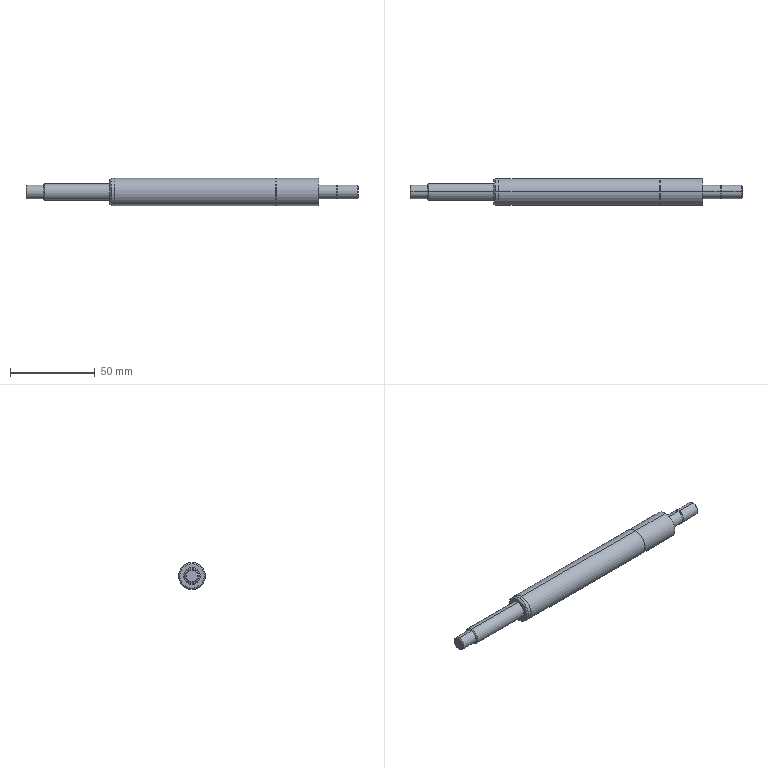Part | SolidWorks | features Chamfer 2, RevCut 1, Revolution 1 | 1 solid | 39 faces | box 196 x 16 x 16 mm | volume 29474 mm3 | cylinder 20 | plane 11 | cone 8 | commonest cylinder face diameters 8 x6 16 x6 12.8 x4 7.6 x2 10 x2
STEP:
#1=CARTESIAN_POINT('',(49.5,0.,7.2));
#2=VERTEX_POINT('',#1);
#3=CARTESIAN_POINT('',(49.5,0.,-7.2));
#4=VERTEX_POINT('',#3);
#5=CARTESIAN_POINT('',(49.5,0.,0.));
#6=DIRECTION('',(-1.,0.,0.));
#7=DIRECTION('',(0.,0.,1.));
#8=AXIS2_PLACEMENT_3D('',#5,#6,#7);
#9=CIRCLE('',#8,7.2);
#10=EDGE_CURVE('',#2,#4,#9,.T.);
#11=ORIENTED_EDGE('',*,*,#10,.F.);
#12=CARTESIAN_POINT('',(50.3,0.,8.));
#13=VERTEX_POINT('',#12);
#14=CARTESIAN_POINT('',(49.5,0.,7.2));
#15=DIRECTION('',(0.7071,0.,0.7071));
#16=VECTOR('',#15,1000.);
#17=LINE('',#14,#16);
#18=EDGE_CURVE('',#2,#13,#17,.T.);
#19=ORIENTED_EDGE('',*,*,#18,.T.);
#20=CARTESIAN_POINT('',(50.3,0.,-8.));
#21=VERTEX_POINT('',#20);
#22=CARTESIAN_POINT('',(50.3,0.,0.));
#23=DIRECTION('',(1.,0.,0.));
#24=DIRECTION('',(0.,0.,1.));
#25=AXIS2_PLACEMENT_3D('',#22,#23,#24);
#26=CIRCLE('',#25,8.);
#27=EDGE_CURVE('',#21,#13,#26,.T.);
#28=ORIENTED_EDGE('',*,*,#27,.F.);
#29=CARTESIAN_POINT('',(49.5,0.,-7.2));
#30=DIRECTION('',(0.7071,0.,-0.7071));
#31=VECTOR('',#30,1000.);
#32=LINE('',#29,#31);
#33=EDGE_CURVE('',#4,#21,#32,.T.);
#34=ORIENTED_EDGE('',*,*,#33,.F.);
#35=EDGE_LOOP('',(#11,#19,#28,#34));
#36=FACE_OUTER_BOUND('',#35,.T.);
#37=CARTESIAN_POINT('',(49.5,0.,0.));
#38=DIRECTION('',(1.,0.,0.));
#39=DIRECTION('',(0.,0.,-1.));
#40=AXIS2_PLACEMENT_3D('',#37,#38,#39);
#41=CONICAL_SURFACE('',#40,7.2,0.7854);
#42=ADVANCED_FACE('',(#36),#41,.T.);
#43=CARTESIAN_POINT('',(196.,0.,-3.5));
#44=VERTEX_POINT('',#43);
#45=CARTESIAN_POINT('',(196.,0.,3.5));
#46=VERTEX_POINT('',#45);
#47=CARTESIAN_POINT('',(196.,0.,0.));
#48=DIRECTION('',(1.,0.,0.));
#49=DIRECTION('',(0.,0.,-1.));
#50=AXIS2_PLACEMENT_3D('',#47,#48,#49);
#51=CIRCLE('',#50,3.5);
#52=EDGE_CURVE('',#44,#46,#51,.T.);
#53=ORIENTED_EDGE('',*,*,#52,.F.);
#54=CARTESIAN_POINT('',(195.5,0.,-4.));
#55=VERTEX_POINT('',#54);
#56=CARTESIAN_POINT('',(195.5,0.,-4.));
#57=DIRECTION('',(-0.7071,0.,-0.7071));
#58=VECTOR('',#57,1000.);
#59=LINE('',#56,#58);
#60=EDGE_CURVE('',#44,#55,#59,.T.);
#61=ORIENTED_EDGE('',*,*,#60,.T.);
#62=CARTESIAN_POINT('',(195.5,0.,4.));
#63=VERTEX_POINT('',#62);
#64=CARTESIAN_POINT('',(195.5,0.,0.));
#65=DIRECTION('',(-1.,0.,0.));
#66=DIRECTION('',(0.,0.,-1.));
#67=AXIS2_PLACEMENT_3D('',#64,#65,#66);
#68=CIRCLE('',#67,4.);
#69=EDGE_CURVE('',#63,#55,#68,.T.);
#70=ORIENTED_EDGE('',*,*,#69,.F.);
#71=CARTESIAN_POINT('',(195.5,0.,4.));
#72=DIRECTION('',(-0.7071,0.,0.7071));
#73=VECTOR('',#72,1000.);
#74=LINE('',#71,#73);
#75=EDGE_CURVE('',#46,#63,#74,.T.);
#76=ORIENTED_EDGE('',*,*,#75,.F.);
#77=EDGE_LOOP('',(#53,#61,#70,#76));
#78=FACE_OUTER_BOUND('',#77,.T.);
#79=CARTESIAN_POINT('',(195.5,0.,0.));
#80=DIRECTION('',(-1.,0.,0.));
#81=DIRECTION('',(0.,0.,1.));
#82=AXIS2_PLACEMENT_3D('',#79,#80,#81);
#83=CONICAL_SURFACE('',#82,4.,0.7854);
#84=ADVANCED_FACE('',(#78),#83,.T.);
#85=CARTESIAN_POINT('',(0.,0.,3.5));
#86=VERTEX_POINT('',#85);
#87=CARTESIAN_POINT('',(0.,0.,-3.5));
#88=VERTEX_POINT('',#87);
#89=CARTESIAN_POINT('',(0.,0.,0.));
#90=DIRECTION('',(-1.,0.,0.));
#91=DIRECTION('',(0.,0.,1.));
#92=AXIS2_PLACEMENT_3D('',#89,#90,#91);
#93=CIRCLE('',#92,3.5);
#94=EDGE_CURVE('',#86,#88,#93,.T.);
#95=ORIENTED_EDGE('',*,*,#94,.F.);
#96=CARTESIAN_POINT('',(0.5,0.,4.));
#97=VERTEX_POINT('',#96);
#98=CARTESIAN_POINT('',(0.,0.,3.5));
#99=DIRECTION('',(0.7071,0.,0.7071));
#100=VECTOR('',#99,1000.);
#101=LINE('',#98,#100);
#102=EDGE_CURVE('',#86,#97,#101,.T.);
#103=ORIENTED_EDGE('',*,*,#102,.T.);
#104=CARTESIAN_POINT('',(0.5,0.,-4.));
#105=VERTEX_POINT('',#104);
#106=CARTESIAN_POINT('',(0.5,0.,0.));
#107=DIRECTION('',(1.,0.,0.));
#108=DIRECTION('',(0.,0.,1.));
#109=AXIS2_PLACEMENT_3D('',#106,#107,#108);
#110=CIRCLE('',#109,4.);
#111=EDGE_CURVE('',#105,#97,#110,.T.);
#112=ORIENTED_EDGE('',*,*,#111,.F.);
#113=CARTESIAN_POINT('',(0.,0.,-3.5));
#114=DIRECTION('',(0.7071,0.,-0.7071));
#115=VECTOR('',#114,1000.);
#116=LINE('',#113,#115);
#117=EDGE_CURVE('',#88,#105,#116,.T.);
#118=ORIENTED_EDGE('',*,*,#117,.F.);
#119=EDGE_LOOP('',(#95,#103,#112,#118));
#120=FACE_OUTER_BOUND('',#119,.T.);
#121=CARTESIAN_POINT('',(0.,0.,0.));
#122=DIRECTION('',(1.,0.,0.));
#123=DIRECTION('',(0.,0.,-1.));
#124=AXIS2_PLACEMENT_3D('',#121,#122,#123);
#125=CONICAL_SURFACE('',#124,3.5,0.7854);
#126=ADVANCED_FACE('',(#120),#125,.T.);
#127=CARTESIAN_POINT('',(10.5,0.,4.5));
#128=VERTEX_POINT('',#127);
#129=CARTESIAN_POINT('',(10.5,0.,-4.5));
#130=VERTEX_POINT('',#129);
#131=CARTESIAN_POINT('',(10.5,0.,0.));
#132=DIRECTION('',(-1.,0.,0.));
#133=DIRECTION('',(0.,0.,1.));
#134=AXIS2_PLACEMENT_3D('',#131,#132,#133);
#135=CIRCLE('',#134,4.5);
#136=EDGE_CURVE('',#128,#130,#135,.T.);
#137=ORIENTED_EDGE('',*,*,#136,.F.);
#138=CARTESIAN_POINT('',(11.,0.,5.));
#139=VERTEX_POINT('',#138);
#140=CARTESIAN_POINT('',(10.5,0.,4.5));
#141=DIRECTION('',(0.7071,0.,0.7071));
#142=VECTOR('',#141,1000.);
#143=LINE('',#140,#142);
#144=EDGE_CURVE('',#128,#139,#143,.T.);
#145=ORIENTED_EDGE('',*,*,#144,.T.);
#146=CARTESIAN_POINT('',(11.,0.,-5.));
#147=VERTEX_POINT('',#146);
#148=CARTESIAN_POINT('',(11.,0.,0.));
#149=DIRECTION('',(1.,0.,0.));
#150=DIRECTION('',(0.,0.,1.));
#151=AXIS2_PLACEMENT_3D('',#148,#149,#150);
#152=CIRCLE('',#151,5.);
#153=EDGE_CURVE('',#147,#139,#152,.T.);
#154=ORIENTED_EDGE('',*,*,#153,.F.);
#155=CARTESIAN_POINT('',(10.5,0.,-4.5));
#156=DIRECTION('',(0.7071,0.,-0.7071));
#157=VECTOR('',#156,1000.);
#158=LINE('',#155,#157);
#159=EDGE_CURVE('',#130,#147,#158,.T.);
#160=ORIENTED_EDGE('',*,*,#159,.F.);
#161=EDGE_LOOP('',(#137,#145,#154,#160));
#162=FACE_OUTER_BOUND('',#161,.T.);
#163=CARTESIAN_POINT('',(10.5,0.,0.));
#164=DIRECTION('',(1.,0.,0.));
#165=DIRECTION('',(0.,0.,-1.));
#166=AXIS2_PLACEMENT_3D('',#163,#164,#165);
#167=CONICAL_SURFACE('',#166,4.5,0.7854);
#168=ADVANCED_FACE('',(#162),#167,.T.);
#169=ORIENTED_EDGE('',*,*,#69,.T.);
#170=CARTESIAN_POINT('',(184.,0.,-4.));
#171=VERTEX_POINT('',#170);
#172=CARTESIAN_POINT('',(-12.257,0.,-4.));
#173=DIRECTION('',(-1.,0.,0.));
#174=VECTOR('',#173,1000.);
#175=LINE('',#172,#174);
#176=EDGE_CURVE('',#55,#171,#175,.T.);
#177=ORIENTED_EDGE('',*,*,#176,.T.);
#178=CARTESIAN_POINT('',(184.,0.,4.));
#179=VERTEX_POINT('',#178);
#180=CARTESIAN_POINT('',(184.,0.,0.));
#181=DIRECTION('',(-1.,0.,0.));
#182=DIRECTION('',(0.,0.,1.));
#183=AXIS2_PLACEMENT_3D('',#180,#181,#182);
#184=CIRCLE('',#183,4.);
#185=EDGE_CURVE('',#179,#171,#184,.T.);
#186=ORIENTED_EDGE('',*,*,#185,.F.);
#187=CARTESIAN_POINT('',(-12.257,0.,4.));
#188=DIRECTION('',(-1.,0.,0.));
#189=VECTOR('',#188,1000.);
#190=LINE('',#187,#189);
#191=EDGE_CURVE('',#63,#179,#190,.T.);
#192=ORIENTED_EDGE('',*,*,#191,.F.);
#193=EDGE_LOOP('',(#169,#177,#186,#192));
#194=FACE_OUTER_BOUND('',#193,.T.);
#195=CARTESIAN_POINT('',(-12.257,0.,0.));
#196=DIRECTION('',(-1.,0.,0.));
#197=DIRECTION('',(0.,0.,1.));
#198=AXIS2_PLACEMENT_3D('',#195,#196,#197);
#199=CYLINDRICAL_SURFACE('',#198,4.);
#200=ADVANCED_FACE('',(#194),#199,.T.);
#201=CARTESIAN_POINT('',(184.,0.,3.8));
#202=VERTEX_POINT('',#201);
#203=CARTESIAN_POINT('',(184.,0.,-3.8));
#204=VERTEX_POINT('',#203);
#205=CARTESIAN_POINT('',(184.,0.,0.));
#206=DIRECTION('',(-1.,0.,0.));
#207=DIRECTION('',(0.,0.,1.));
#208=AXIS2_PLACEMENT_3D('',#205,#206,#207);
#209=CIRCLE('',#208,3.8);
#210=EDGE_CURVE('',#202,#204,#209,.T.);
#211=ORIENTED_EDGE('',*,*,#210,.T.);
#212=CARTESIAN_POINT('',(183.1,0.,-3.8));
#213=VERTEX_POINT('',#212);
#214=CARTESIAN_POINT('',(-6.355,0.,-3.8));
#215=DIRECTION('',(-1.,0.,0.));
#216=VECTOR('',#215,1000.);
#217=LINE('',#214,#216);
#218=EDGE_CURVE('',#204,#213,#217,.T.);
#219=ORIENTED_EDGE('',*,*,#218,.T.);
#220=CARTESIAN_POINT('',(183.1,0.,3.8));
#221=VERTEX_POINT('',#220);
#222=CARTESIAN_POINT('',(183.1,0.,0.));
#223=DIRECTION('',(-1.,0.,0.));
#224=DIRECTION('',(0.,0.,1.));
#225=AXIS2_PLACEMENT_3D('',#222,#223,#224);
#226=CIRCLE('',#225,3.8);
#227=EDGE_CURVE('',#221,#213,#226,.T.);
#228=ORIENTED_EDGE('',*,*,#227,.F.);
#229=CARTESIAN_POINT('',(-6.355,0.,3.8));
#230=DIRECTION('',(-1.,0.,0.));
#231=VECTOR('',#230,1000.);
#232=LINE('',#229,#231);
#233=EDGE_CURVE('',#202,#221,#232,.T.);
#234=ORIENTED_EDGE('',*,*,#233,.F.);
#235=EDGE_LOOP('',(#211,#219,#228,#234));
#236=FACE_OUTER_BOUND('',#235,.T.);
#237=CARTESIAN_POINT('',(-6.355,0.,0.));
#238=DIRECTION('',(-1.,0.,0.));
#239=DIRECTION('',(0.,0.,1.));
#240=AXIS2_PLACEMENT_3D('',#237,#238,#239);
#241=CYLINDRICAL_SURFACE('',#240,3.8);
#242=ADVANCED_FACE('',(#236),#241,.T.);
#243=CARTESIAN_POINT('',(172.7,0.,8.));
#244=VERTEX_POINT('',#243);
#245=CARTESIAN_POINT('',(172.7,0.,-8.));
#246=VERTEX_POINT('',#245);
#247=CARTESIAN_POINT('',(172.7,0.,0.));
#248=DIRECTION('',(-1.,0.,0.));
#249=DIRECTION('',(0.,0.,1.));
#250=AXIS2_PLACEMENT_3D('',#247,#248,#249);
#251=CIRCLE('',#250,8.);
#252=EDGE_CURVE('',#244,#246,#251,.T.);
#253=ORIENTED_EDGE('',*,*,#252,.T.);
#254=CARTESIAN_POINT('',(147.7,0.,-8.));
#255=VERTEX_POINT('',#254);
#256=CARTESIAN_POINT('',(-12.257,0.,-8.));
#257=DIRECTION('',(-1.,0.,0.));
#258=VECTOR('',#257,1000.);
#259=LINE('',#256,#258);
#260=EDGE_CURVE('',#246,#255,#259,.T.);
#261=ORIENTED_EDGE('',*,*,#260,.T.);
#262=CARTESIAN_POINT('',(147.7,0.,8.));
#263=VERTEX_POINT('',#262);
#264=CARTESIAN_POINT('',(147.7,0.,0.));
#265=DIRECTION('',(-1.,0.,0.));
#266=DIRECTION('',(0.,0.,1.));
#267=AXIS2_PLACEMENT_3D('',#264,#265,#266);
#268=CIRCLE('',#267,8.);
#269=EDGE_CURVE('',#263,#255,#268,.T.);
#270=ORIENTED_EDGE('',*,*,#269,.F.);
#271=CARTESIAN_POINT('',(-12.257,0.,8.));
#272=DIRECTION('',(-1.,0.,0.));
#273=VECTOR('',#272,1000.);
#274=LINE('',#271,#273);
#275=EDGE_CURVE('',#244,#263,#274,.T.);
#276=ORIENTED_EDGE('',*,*,#275,.F.);
#277=EDGE_LOOP('',(#253,#261,#270,#276));
#278=FACE_OUTER_BOUND('',#277,.T.);
#279=CARTESIAN_POINT('',(-12.257,0.,0.));
#280=DIRECTION('',(-1.,0.,0.));
#281=DIRECTION('',(0.,0.,1.));
#282=AXIS2_PLACEMENT_3D('',#279,#280,#281);
#283=CYLINDRICAL_SURFACE('',#282,8.);
#284=ADVANCED_FACE('',(#278),#283,.T.);
#285=CARTESIAN_POINT('',(147.7,0.,6.4));
#286=VERTEX_POINT('',#285);
#287=CARTESIAN_POINT('',(147.7,0.,-6.4));
#288=VERTEX_POINT('',#287);
#289=CARTESIAN_POINT('',(147.7,0.,0.));
#290=DIRECTION('',(-1.,0.,0.));
#291=DIRECTION('',(0.,0.,1.));
#292=AXIS2_PLACEMENT_3D('',#289,#290,#291);
#293=CIRCLE('',#292,6.4);
#294=EDGE_CURVE('',#286,#288,#293,.T.);
#295=ORIENTED_EDGE('',*,*,#294,.T.);
#296=CARTESIAN_POINT('',(147.5,0.,-6.4));
#297=VERTEX_POINT('',#296);
#298=CARTESIAN_POINT('',(-6.355,0.,-6.4));
#299=DIRECTION('',(-1.,0.,0.));
#300=VECTOR('',#299,1000.);
#301=LINE('',#298,#300);
#302=EDGE_CURVE('',#288,#297,#301,.T.);
#303=ORIENTED_EDGE('',*,*,#302,.T.);
#304=CARTESIAN_POINT('',(147.5,0.,6.4));
#305=VERTEX_POINT('',#304);
#306=CARTESIAN_POINT('',(147.5,0.,0.));
#307=DIRECTION('',(-1.,0.,0.));
#308=DIRECTION('',(0.,0.,1.));
#309=AXIS2_PLACEMENT_3D('',#306,#307,#308);
#310=CIRCLE('',#309,6.4);
#311=EDGE_CURVE('',#305,#297,#310,.T.);
#312=ORIENTED_EDGE('',*,*,#311,.F.);
#313=CARTESIAN_POINT('',(-6.355,0.,6.4));
#314=DIRECTION('',(-1.,0.,0.));
#315=VECTOR('',#314,1000.);
#316=LINE('',#313,#315);
#317=EDGE_CURVE('',#286,#305,#316,.T.);
#318=ORIENTED_EDGE('',*,*,#317,.F.);
#319=EDGE_LOOP('',(#295,#303,#312,#318));
#320=FACE_OUTER_BOUND('',#319,.T.);
#321=CARTESIAN_POINT('',(-6.355,0.,0.));
#322=DIRECTION('',(-1.,0.,0.));
#323=DIRECTION('',(0.,0.,1.));
#324=AXIS2_PLACEMENT_3D('',#321,#322,#323);
#325=CYLINDRICAL_SURFACE('',#324,6.4);
#326=ADVANCED_FACE('',(#320),#325,.T.);
#327=CARTESIAN_POINT('',(52.5,0.,6.4));
#328=VERTEX_POINT('',#327);
#329=CARTESIAN_POINT('',(52.5,0.,-6.4));
#330=VERTEX_POINT('',#329);
#331=CARTESIAN_POINT('',(52.5,0.,0.));
#332=DIRECTION('',(-1.,0.,0.));
#333=DIRECTION('',(0.,0.,1.));
#334=AXIS2_PLACEMENT_3D('',#331,#332,#333);
#335=CIRCLE('',#334,6.4);
#336=EDGE_CURVE('',#328,#330,#335,.T.);
#337=ORIENTED_EDGE('',*,*,#336,.T.);
#338=CARTESIAN_POINT('',(52.3,0.,-6.4));
#339=VERTEX_POINT('',#338);
#340=CARTESIAN_POINT('',(-6.355,0.,-6.4));
#341=DIRECTION('',(-1.,0.,0.));
#342=VECTOR('',#341,1000.);
#343=LINE('',#340,#342);
#344=EDGE_CURVE('',#330,#339,#343,.T.);
#345=ORIENTED_EDGE('',*,*,#344,.T.);
#346=CARTESIAN_POINT('',(52.3,0.,6.4));
#347=VERTEX_POINT('',#346);
#348=CARTESIAN_POINT('',(52.3,0.,0.));
#349=DIRECTION('',(-1.,0.,0.));
#350=DIRECTION('',(0.,0.,1.));
#351=AXIS2_PLACEMENT_3D('',#348,#349,#350);
#352=CIRCLE('',#351,6.4);
#353=EDGE_CURVE('',#347,#339,#352,.T.);
#354=ORIENTED_EDGE('',*,*,#353,.F.);
#355=CARTESIAN_POINT('',(-6.355,0.,6.4));
#356=DIRECTION('',(-1.,0.,0.));
#357=VECTOR('',#356,1000.);
#358=LINE('',#355,#357);
#359=EDGE_CURVE('',#328,#347,#358,.T.);
#360=ORIENTED_EDGE('',*,*,#359,.F.);
#361=EDGE_LOOP('',(#337,#345,#354,#360));
#362=FACE_OUTER_BOUND('',#361,.T.);
#363=CARTESIAN_POINT('',(-6.355,0.,0.));
#364=DIRECTION('',(-1.,0.,0.));
#365=DIRECTION('',(0.,0.,1.));
#366=AXIS2_PLACEMENT_3D('',#363,#364,#365);
#367=CYLINDRICAL_SURFACE('',#366,6.4);
#368=ADVANCED_FACE('',(#362),#367,.T.);
#369=CARTESIAN_POINT('',(49.5,0.,5.));
#370=VERTEX_POINT('',#369);
#371=CARTESIAN_POINT('',(49.5,0.,-5.));
#372=VERTEX_POINT('',#371);
#373=CARTESIAN_POINT('',(49.5,0.,0.));
#374=DIRECTION('',(-1.,0.,0.));
#375=DIRECTION('',(0.,0.,1.));
#376=AXIS2_PLACEMENT_3D('',#373,#374,#375);
#377=CIRCLE('',#376,5.);
#378=EDGE_CURVE('',#370,#372,#377,.T.);
#379=ORIENTED_EDGE('',*,*,#378,.T.);
#380=CARTESIAN_POINT('',(-12.257,0.,-5.));
#381=DIRECTION('',(-1.,0.,0.));
#382=VECTOR('',#381,1000.);
#383=LINE('',#380,#382);
#384=EDGE_CURVE('',#372,#147,#383,.T.);
#385=ORIENTED_EDGE('',*,*,#384,.T.);
#386=ORIENTED_EDGE('',*,*,#153,.T.);
#387=CARTESIAN_POINT('',(-12.257,0.,5.));
#388=DIRECTION('',(-1.,0.,0.));
#389=VECTOR('',#388,1000.);
#390=LINE('',#387,#389);
#391=EDGE_CURVE('',#370,#139,#390,.T.);
#392=ORIENTED_EDGE('',*,*,#391,.F.);
#393=EDGE_LOOP('',(#379,#385,#386,#392));
#394=FACE_OUTER_BOUND('',#393,.T.);
#395=CARTESIAN_POINT('',(-12.257,0.,0.));
#396=DIRECTION('',(-1.,0.,0.));
#397=DIRECTION('',(0.,0.,1.));
#398=AXIS2_PLACEMENT_3D('',#395,#396,#397);
#399=CYLINDRICAL_SURFACE('',#398,5.);
#400=ADVANCED_FACE('',(#394),#399,.T.);
#401=CARTESIAN_POINT('',(10.5,0.,4.));
#402=VERTEX_POINT('',#401);
#403=CARTESIAN_POINT('',(10.5,0.,-4.));
#404=VERTEX_POINT('',#403);
#405=CARTESIAN_POINT('',(10.5,0.,0.));
#406=DIRECTION('',(-1.,0.,0.));
#407=DIRECTION('',(0.,0.,1.));
#408=AXIS2_PLACEMENT_3D('',#405,#406,#407);
#409=CIRCLE('',#408,4.);
#410=EDGE_CURVE('',#402,#404,#409,.T.);
#411=ORIENTED_EDGE('',*,*,#410,.T.);
#412=CARTESIAN_POINT('',(-12.257,0.,-4.));
#413=DIRECTION('',(-1.,0.,0.));
#414=VECTOR('',#413,1000.);
#415=LINE('',#412,#414);
#416=EDGE_CURVE('',#404,#105,#415,.T.);
#417=ORIENTED_EDGE('',*,*,#416,.T.);
#418=ORIENTED_EDGE('',*,*,#111,.T.);
#419=CARTESIAN_POINT('',(-12.257,0.,4.));
#420=DIRECTION('',(-1.,0.,0.));
#421=VECTOR('',#420,1000.);
#422=LINE('',#419,#421);
#423=EDGE_CURVE('',#402,#97,#422,.T.);
#424=ORIENTED_EDGE('',*,*,#423,.F.);
#425=EDGE_LOOP('',(#411,#417,#418,#424));
#426=FACE_OUTER_BOUND('',#425,.T.);
#427=CARTESIAN_POINT('',(-12.257,0.,0.));
#428=DIRECTION('',(-1.,0.,0.));
#429=DIRECTION('',(0.,0.,1.));
#430=AXIS2_PLACEMENT_3D('',#427,#428,#429);
#431=CYLINDRICAL_SURFACE('',#430,4.);
#432=ADVANCED_FACE('',(#426),#431,.T.);
#433=CARTESIAN_POINT('',(52.3,0.,8.));
#434=VERTEX_POINT('',#433);
#435=CARTESIAN_POINT('',(52.3,0.,-8.));
#436=VERTEX_POINT('',#435);
#437=CARTESIAN_POINT('',(52.3,0.,0.));
#438=DIRECTION('',(-1.,0.,0.));
#439=DIRECTION('',(0.,0.,1.));
#440=AXIS2_PLACEMENT_3D('',#437,#438,#439);
#441=CIRCLE('',#440,8.);
#442=EDGE_CURVE('',#434,#436,#441,.T.);
#443=ORIENTED_EDGE('',*,*,#442,.T.);
#444=CARTESIAN_POINT('',(-12.257,0.,-8.));
#445=DIRECTION('',(-1.,0.,0.));
#446=VECTOR('',#445,1000.);
#447=LINE('',#444,#446);
#448=EDGE_CURVE('',#436,#21,#447,.T.);
#449=ORIENTED_EDGE('',*,*,#448,.T.);
#450=ORIENTED_EDGE('',*,*,#27,.T.);
#451=CARTESIAN_POINT('',(-12.257,0.,8.));
#452=DIRECTION('',(-1.,0.,0.));
#453=VECTOR('',#452,1000.);
#454=LINE('',#451,#453);
#455=EDGE_CURVE('',#434,#13,#454,.T.);
#456=ORIENTED_EDGE('',*,*,#455,.F.);
#457=EDGE_LOOP('',(#443,#449,#450,#456));
#458=FACE_OUTER_BOUND('',#457,.T.);
#459=CARTESIAN_POINT('',(-12.257,0.,0.));
#460=DIRECTION('',(-1.,0.,0.));
#461=DIRECTION('',(0.,0.,1.));
#462=AXIS2_PLACEMENT_3D('',#459,#460,#461);
#463=CYLINDRICAL_SURFACE('',#462,8.);
#464=ADVANCED_FACE('',(#458),#463,.T.);
#465=CARTESIAN_POINT('',(147.5,0.,8.));
#466=VERTEX_POINT('',#465);
#467=CARTESIAN_POINT('',(147.5,0.,-8.));
#468=VERTEX_POINT('',#467);
#469=CARTESIAN_POINT('',(147.5,0.,0.));
#470=DIRECTION('',(-1.,0.,0.));
#471=DIRECTION('',(0.,0.,1.));
#472=AXIS2_PLACEMENT_3D('',#469,#470,#471);
#473=CIRCLE('',#472,8.);
#474=EDGE_CURVE('',#466,#468,#473,.T.);
#475=ORIENTED_EDGE('',*,*,#474,.T.);
#476=CARTESIAN_POINT('',(52.5,0.,-8.));
#477=VERTEX_POINT('',#476);
#478=CARTESIAN_POINT('',(-12.257,0.,-8.));
#479=DIRECTION('',(-1.,0.,0.));
#480=VECTOR('',#479,1000.);
#481=LINE('',#478,#480);
#482=EDGE_CURVE('',#468,#477,#481,.T.);
#483=ORIENTED_EDGE('',*,*,#482,.T.);
#484=CARTESIAN_POINT('',(52.5,0.,8.));
#485=VERTEX_POINT('',#484);
#486=CARTESIAN_POINT('',(52.5,0.,0.));
#487=DIRECTION('',(-1.,0.,0.));
#488=DIRECTION('',(0.,0.,1.));
#489=AXIS2_PLACEMENT_3D('',#486,#487,#488);
#490=CIRCLE('',#489,8.);
#491=EDGE_CURVE('',#485,#477,#490,.T.);
#492=ORIENTED_EDGE('',*,*,#491,.F.);
#493=CARTESIAN_POINT('',(-12.257,0.,8.));
#494=DIRECTION('',(-1.,0.,0.));
#495=VECTOR('',#494,1000.);
#496=LINE('',#493,#495);
#497=EDGE_CURVE('',#466,#485,#496,.T.);
#498=ORIENTED_EDGE('',*,*,#497,.F.);
#499=EDGE_LOOP('',(#475,#483,#492,#498));
#500=FACE_OUTER_BOUND('',#499,.T.);
#501=CARTESIAN_POINT('',(-12.257,0.,0.));
#502=DIRECTION('',(-1.,0.,0.));
#503=DIRECTION('',(0.,0.,1.));
#504=AXIS2_PLACEMENT_3D('',#501,#502,#503);
#505=CYLINDRICAL_SURFACE('',#504,8.);
#506=ADVANCED_FACE('',(#500),#505,.T.);
#507=CARTESIAN_POINT('',(183.1,0.,4.));
#508=VERTEX_POINT('',#507);
#509=CARTESIAN_POINT('',(183.1,0.,-4.));
#510=VERTEX_POINT('',#509);
#511=CARTESIAN_POINT('',(183.1,0.,0.));
#512=DIRECTION('',(-1.,0.,0.));
#513=DIRECTION('',(0.,0.,1.));
#514=AXIS2_PLACEMENT_3D('',#511,#512,#513);
#515=CIRCLE('',#514,4.);
#516=EDGE_CURVE('',#508,#510,#515,.T.);
#517=ORIENTED_EDGE('',*,*,#516,.T.);
#518=CARTESIAN_POINT('',(172.7,0.,-4.));
#519=VERTEX_POINT('',#518);
#520=CARTESIAN_POINT('',(-12.257,0.,-4.));
#521=DIRECTION('',(-1.,0.,0.));
#522=VECTOR('',#521,1000.);
#523=LINE('',#520,#522);
#524=EDGE_CURVE('',#510,#519,#523,.T.);
#525=ORIENTED_EDGE('',*,*,#524,.T.);
#526=CARTESIAN_POINT('',(172.7,0.,4.));
#527=VERTEX_POINT('',#526);
#528=CARTESIAN_POINT('',(172.7,0.,0.));
#529=DIRECTION('',(-1.,0.,0.));
#530=DIRECTION('',(0.,0.,1.));
#531=AXIS2_PLACEMENT_3D('',#528,#529,#530);
#532=CIRCLE('',#531,4.);
#533=EDGE_CURVE('',#527,#519,#532,.T.);
#534=ORIENTED_EDGE('',*,*,#533,.F.);
#535=CARTESIAN_POINT('',(-12.257,0.,4.));
#536=DIRECTION('',(-1.,0.,0.));
#537=VECTOR('',#536,1000.);
#538=LINE('',#535,#537);
#539=EDGE_CURVE('',#508,#527,#538,.T.);
#540=ORIENTED_EDGE('',*,*,#539,.F.);
#541=EDGE_LOOP('',(#517,#525,#534,#540));
#542=FACE_OUTER_BOUND('',#541,.T.);
#543=CARTESIAN_POINT('',(-12.257,0.,0.));
#544=DIRECTION('',(-1.,0.,0.));
#545=DIRECTION('',(0.,0.,1.));
#546=AXIS2_PLACEMENT_3D('',#543,#544,#545);
#547=CYLINDRICAL_SURFACE('',#546,4.);
#548=ADVANCED_FACE('',(#542),#547,.T.);
#549=ORIENTED_EDGE('',*,*,#524,.F.);
#550=CARTESIAN_POINT('',(183.1,0.,0.));
#551=DIRECTION('',(-1.,0.,0.));
#552=DIRECTION('',(0.,0.,1.));
#553=AXIS2_PLACEMENT_3D('',#550,#551,#552);
#554=CIRCLE('',#553,4.);
#555=EDGE_CURVE('',#510,#508,#554,.T.);
#556=ORIENTED_EDGE('',*,*,#555,.T.);
#557=ORIENTED_EDGE('',*,*,#539,.T.);
#558=CARTESIAN_POINT('',(172.7,0.,0.));
#559=DIRECTION('',(-1.,0.,0.));
#560=DIRECTION('',(0.,0.,1.));
#561=AXIS2_PLACEMENT_3D('',#558,#559,#560);
#562=CIRCLE('',#561,4.);
#563=EDGE_CURVE('',#519,#527,#562,.T.);
#564=ORIENTED_EDGE('',*,*,#563,.F.);
#565=EDGE_LOOP('',(#549,#556,#557,#564));
#566=FACE_OUTER_BOUND('',#565,.T.);
#567=CARTESIAN_POINT('',(-12.257,0.,0.));
#568=DIRECTION('',(-1.,0.,0.));
#569=DIRECTION('',(0.,0.,1.));
#570=AXIS2_PLACEMENT_3D('',#567,#568,#569);
#571=CYLINDRICAL_SURFACE('',#570,4.);
#572=ADVANCED_FACE('',(#566),#571,.T.);
#573=ORIENTED_EDGE('',*,*,#482,.F.);
#574=CARTESIAN_POINT('',(147.5,0.,0.));
#575=DIRECTION('',(-1.,0.,0.));
#576=DIRECTION('',(0.,0.,1.));
#577=AXIS2_PLACEMENT_3D('',#574,#575,#576);
#578=CIRCLE('',#577,8.);
#579=EDGE_CURVE('',#468,#466,#578,.T.);
#580=ORIENTED_EDGE('',*,*,#579,.T.);
#581=ORIENTED_EDGE('',*,*,#497,.T.);
#582=CARTESIAN_POINT('',(52.5,0.,0.));
#583=DIRECTION('',(-1.,0.,0.));
#584=DIRECTION('',(0.,0.,1.));
#585=AXIS2_PLACEMENT_3D('',#582,#583,#584);
#586=CIRCLE('',#585,8.);
#587=EDGE_CURVE('',#477,#485,#586,.T.);
#588=ORIENTED_EDGE('',*,*,#587,.F.);
#589=EDGE_LOOP('',(#573,#580,#581,#588));
#590=FACE_OUTER_BOUND('',#589,.T.);
#591=CARTESIAN_POINT('',(-12.257,0.,0.));
#592=DIRECTION('',(-1.,0.,0.));
#593=DIRECTION('',(0.,0.,1.));
#594=AXIS2_PLACEMENT_3D('',#591,#592,#593);
#595=CYLINDRICAL_SURFACE('',#594,8.);
#596=ADVANCED_FACE('',(#590),#595,.T.);
#597=ORIENTED_EDGE('',*,*,#448,.F.);
#598=CARTESIAN_POINT('',(52.3,0.,0.));
#599=DIRECTION('',(-1.,0.,0.));
#600=DIRECTION('',(0.,0.,1.));
#601=AXIS2_PLACEMENT_3D('',#598,#599,#600);
#602=CIRCLE('',#601,8.);
#603=EDGE_CURVE('',#436,#434,#602,.T.);
#604=ORIENTED_EDGE('',*,*,#603,.T.);
#605=ORIENTED_EDGE('',*,*,#455,.T.);
#606=CARTESIAN_POINT('',(50.3,0.,0.));
#607=DIRECTION('',(1.,0.,0.));
#608=DIRECTION('',(0.,0.,1.));
#609=AXIS2_PLACEMENT_3D('',#606,#607,#608);
#610=CIRCLE('',#609,8.);
#611=EDGE_CURVE('',#13,#21,#610,.T.);
#612=ORIENTED_EDGE('',*,*,#611,.T.);
#613=EDGE_LOOP('',(#597,#604,#605,#612));
#614=FACE_OUTER_BOUND('',#613,.T.);
#615=CARTESIAN_POINT('',(-12.257,0.,0.));
#616=DIRECTION('',(-1.,0.,0.));
#617=DIRECTION('',(0.,0.,1.));
#618=AXIS2_PLACEMENT_3D('',#615,#616,#617);
#619=CYLINDRICAL_SURFACE('',#618,8.);
#620=ADVANCED_FACE('',(#614),#619,.T.);
#621=CARTESIAN_POINT('',(0.,0.,0.));
#622=DIRECTION('',(-1.,0.,0.));
#623=DIRECTION('',(0.,0.,1.));
#624=AXIS2_PLACEMENT_3D('',#621,#622,#623);
#625=CIRCLE('',#624,3.5);
#626=EDGE_CURVE('',#88,#86,#625,.T.);
#627=ORIENTED_EDGE('',*,*,#626,.T.);
#628=ORIENTED_EDGE('',*,*,#94,.T.);
#629=EDGE_LOOP('',(#627,#628));
#630=FACE_OUTER_BOUND('',#629,.T.);
#631=CARTESIAN_POINT('',(0.,0.,0.));
#632=DIRECTION('',(-1.,0.,0.));
#633=DIRECTION('',(0.,0.,1.));
#634=AXIS2_PLACEMENT_3D('',#631,#632,#633);
#635=PLANE('',#634);
#636=ADVANCED_FACE('',(#630),#635,.T.);
#637=ORIENTED_EDGE('',*,*,#416,.F.);
#638=CARTESIAN_POINT('',(10.5,0.,0.));
#639=DIRECTION('',(-1.,0.,0.));
#640=DIRECTION('',(0.,0.,1.));
#641=AXIS2_PLACEMENT_3D('',#638,#639,#640);
#642=CIRCLE('',#641,4.);
#643=EDGE_CURVE('',#404,#402,#642,.T.);
#644=ORIENTED_EDGE('',*,*,#643,.T.);
#645=ORIENTED_EDGE('',*,*,#423,.T.);
#646=CARTESIAN_POINT('',(0.5,0.,0.));
#647=DIRECTION('',(1.,0.,0.));
#648=DIRECTION('',(0.,0.,1.));
#649=AXIS2_PLACEMENT_3D('',#646,#647,#648);
#650=CIRCLE('',#649,4.);
#651=EDGE_CURVE('',#97,#105,#650,.T.);
#652=ORIENTED_EDGE('',*,*,#651,.T.);
#653=EDGE_LOOP('',(#637,#644,#645,#652));
#654=FACE_OUTER_BOUND('',#653,.T.);
#655=CARTESIAN_POINT('',(-12.257,0.,0.));
#656=DIRECTION('',(-1.,0.,0.));
#657=DIRECTION('',(0.,0.,1.));
#658=AXIS2_PLACEMENT_3D('',#655,#656,#657);
#659=CYLINDRICAL_SURFACE('',#658,4.);
#660=ADVANCED_FACE('',(#654),#659,.T.);
#661=CARTESIAN_POINT('',(10.5,0.,0.));
#662=DIRECTION('',(-1.,0.,0.));
#663=DIRECTION('',(0.,0.,1.));
#664=AXIS2_PLACEMENT_3D('',#661,#662,#663);
#665=CIRCLE('',#664,4.5);
#666=EDGE_CURVE('',#130,#128,#665,.T.);
#667=ORIENTED_EDGE('',*,*,#666,.T.);
#668=ORIENTED_EDGE('',*,*,#136,.T.);
#669=EDGE_LOOP('',(#667,#668));
#670=FACE_OUTER_BOUND('',#669,.T.);
#671=ORIENTED_EDGE('',*,*,#410,.F.);
#672=ORIENTED_EDGE('',*,*,#643,.F.);
#673=EDGE_LOOP('',(#671,#672));
#674=FACE_BOUND('',#673,.T.);
#675=CARTESIAN_POINT('',(10.5,0.,-4.));
#676=DIRECTION('',(-1.,0.,0.));
#677=DIRECTION('',(0.,0.,1.));
#678=AXIS2_PLACEMENT_3D('',#675,#676,#677);
#679=PLANE('',#678);
#680=ADVANCED_FACE('',(#670,#674),#679,.T.);
#681=ORIENTED_EDGE('',*,*,#384,.F.);
#682=CARTESIAN_POINT('',(49.5,0.,0.));
#683=DIRECTION('',(-1.,0.,0.));
#684=DIRECTION('',(0.,0.,1.));
#685=AXIS2_PLACEMENT_3D('',#682,#683,#684);
#686=CIRCLE('',#685,5.);
#687=EDGE_CURVE('',#372,#370,#686,.T.);
#688=ORIENTED_EDGE('',*,*,#687,.T.);
#689=ORIENTED_EDGE('',*,*,#391,.T.);
#690=CARTESIAN_POINT('',(11.,0.,0.));
#691=DIRECTION('',(1.,0.,0.));
#692=DIRECTION('',(0.,0.,1.));
#693=AXIS2_PLACEMENT_3D('',#690,#691,#692);
#694=CIRCLE('',#693,5.);
#695=EDGE_CURVE('',#139,#147,#694,.T.);
#696=ORIENTED_EDGE('',*,*,#695,.T.);
#697=EDGE_LOOP('',(#681,#688,#689,#696));
#698=FACE_OUTER_BOUND('',#697,.T.);
#699=CARTESIAN_POINT('',(-12.257,0.,0.));
#700=DIRECTION('',(-1.,0.,0.));
#701=DIRECTION('',(0.,0.,1.));
#702=AXIS2_PLACEMENT_3D('',#699,#700,#701);
#703=CYLINDRICAL_SURFACE('',#702,5.);
#704=ADVANCED_FACE('',(#698),#703,.T.);
#705=CARTESIAN_POINT('',(49.5,0.,0.));
#706=DIRECTION('',(-1.,0.,0.));
#707=DIRECTION('',(0.,0.,1.));
#708=AXIS2_PLACEMENT_3D('',#705,#706,#707);
#709=CIRCLE('',#708,7.2);
#710=EDGE_CURVE('',#4,#2,#709,.T.);
#711=ORIENTED_EDGE('',*,*,#710,.T.);
#712=ORIENTED_EDGE('',*,*,#10,.T.);
#713=EDGE_LOOP('',(#711,#712));
#714=FACE_OUTER_BOUND('',#713,.T.);
#715=ORIENTED_EDGE('',*,*,#378,.F.);
#716=ORIENTED_EDGE('',*,*,#687,.F.);
#717=EDGE_LOOP('',(#715,#716));
#718=FACE_BOUND('',#717,.T.);
#719=CARTESIAN_POINT('',(49.5,0.,-5.));
#720=DIRECTION('',(-1.,0.,0.));
#721=DIRECTION('',(0.,0.,1.));
#722=AXIS2_PLACEMENT_3D('',#719,#720,#721);
#723=PLANE('',#722);
#724=ADVANCED_FACE('',(#714,#718),#723,.T.);
#725=ORIENTED_EDGE('',*,*,#442,.F.);
#726=ORIENTED_EDGE('',*,*,#603,.F.);
#727=EDGE_LOOP('',(#725,#726));
#728=FACE_OUTER_BOUND('',#727,.T.);
#729=ORIENTED_EDGE('',*,*,#353,.T.);
#730=CARTESIAN_POINT('',(52.3,0.,0.));
#731=DIRECTION('',(-1.,0.,0.));
#732=DIRECTION('',(0.,0.,1.));
#733=AXIS2_PLACEMENT_3D('',#730,#731,#732);
#734=CIRCLE('',#733,6.4);
#735=EDGE_CURVE('',#339,#347,#734,.T.);
#736=ORIENTED_EDGE('',*,*,#735,.T.);
#737=EDGE_LOOP('',(#729,#736));
#738=FACE_BOUND('',#737,.T.);
#739=CARTESIAN_POINT('',(52.3,0.,-8.));
#740=DIRECTION('',(-1.,0.,0.));
#741=DIRECTION('',(0.,0.,1.));
#742=AXIS2_PLACEMENT_3D('',#739,#740,#741);
#743=PLANE('',#742);
#744=ADVANCED_FACE('',(#728,#738),#743,.F.);
#745=ORIENTED_EDGE('',*,*,#344,.F.);
#746=CARTESIAN_POINT('',(52.5,0.,0.));
#747=DIRECTION('',(-1.,0.,0.));
#748=DIRECTION('',(0.,0.,1.));
#749=AXIS2_PLACEMENT_3D('',#746,#747,#748);
#750=CIRCLE('',#749,6.4);
#751=EDGE_CURVE('',#330,#328,#750,.T.);
#752=ORIENTED_EDGE('',*,*,#751,.T.);
#753=ORIENTED_EDGE('',*,*,#359,.T.);
#754=ORIENTED_EDGE('',*,*,#735,.F.);
#755=EDGE_LOOP('',(#745,#752,#753,#754));
#756=FACE_OUTER_BOUND('',#755,.T.);
#757=CARTESIAN_POINT('',(-6.355,0.,0.));
#758=DIRECTION('',(-1.,0.,0.));
#759=DIRECTION('',(0.,0.,1.));
#760=AXIS2_PLACEMENT_3D('',#757,#758,#759);
#761=CYLINDRICAL_SURFACE('',#760,6.4);
#762=ADVANCED_FACE('',(#756),#761,.T.);
#763=ORIENTED_EDGE('',*,*,#336,.F.);
#764=ORIENTED_EDGE('',*,*,#751,.F.);
#765=EDGE_LOOP('',(#763,#764));
#766=FACE_BOUND('',#765,.T.);
#767=ORIENTED_EDGE('',*,*,#491,.T.);
#768=ORIENTED_EDGE('',*,*,#587,.T.);
#769=EDGE_LOOP('',(#767,#768));
#770=FACE_OUTER_BOUND('',#769,.T.);
#771=CARTESIAN_POINT('',(52.5,0.,-8.));
#772=DIRECTION('',(1.,0.,0.));
#773=DIRECTION('',(0.,0.,-1.));
#774=AXIS2_PLACEMENT_3D('',#771,#772,#773);
#775=PLANE('',#774);
#776=ADVANCED_FACE('',(#766,#770),#775,.F.);
#777=ORIENTED_EDGE('',*,*,#474,.F.);
#778=ORIENTED_EDGE('',*,*,#579,.F.);
#779=EDGE_LOOP('',(#777,#778));
#780=FACE_OUTER_BOUND('',#779,.T.);
#781=ORIENTED_EDGE('',*,*,#311,.T.);
#782=CARTESIAN_POINT('',(147.5,0.,0.));
#783=DIRECTION('',(-1.,0.,0.));
#784=DIRECTION('',(0.,0.,1.));
#785=AXIS2_PLACEMENT_3D('',#782,#783,#784);
#786=CIRCLE('',#785,6.4);
#787=EDGE_CURVE('',#297,#305,#786,.T.);
#788=ORIENTED_EDGE('',*,*,#787,.T.);
#789=EDGE_LOOP('',(#781,#788));
#790=FACE_BOUND('',#789,.T.);
#791=CARTESIAN_POINT('',(147.5,0.,-8.));
#792=DIRECTION('',(-1.,0.,0.));
#793=DIRECTION('',(0.,0.,1.));
#794=AXIS2_PLACEMENT_3D('',#791,#792,#793);
#795=PLANE('',#794);
#796=ADVANCED_FACE('',(#780,#790),#795,.F.);
#797=ORIENTED_EDGE('',*,*,#302,.F.);
#798=CARTESIAN_POINT('',(147.7,0.,0.));
#799=DIRECTION('',(-1.,0.,0.));
#800=DIRECTION('',(0.,0.,1.));
#801=AXIS2_PLACEMENT_3D('',#798,#799,#800);
#802=CIRCLE('',#801,6.4);
#803=EDGE_CURVE('',#288,#286,#802,.T.);
#804=ORIENTED_EDGE('',*,*,#803,.T.);
#805=ORIENTED_EDGE('',*,*,#317,.T.);
#806=ORIENTED_EDGE('',*,*,#787,.F.);
#807=EDGE_LOOP('',(#797,#804,#805,#806));
#808=FACE_OUTER_BOUND('',#807,.T.);
#809=CARTESIAN_POINT('',(-6.355,0.,0.));
#810=DIRECTION('',(-1.,0.,0.));
#811=DIRECTION('',(0.,0.,1.));
#812=AXIS2_PLACEMENT_3D('',#809,#810,#811);
#813=CYLINDRICAL_SURFACE('',#812,6.4);
#814=ADVANCED_FACE('',(#808),#813,.T.);
#815=ORIENTED_EDGE('',*,*,#294,.F.);
#816=ORIENTED_EDGE('',*,*,#803,.F.);
#817=EDGE_LOOP('',(#815,#816));
#818=FACE_BOUND('',#817,.T.);
#819=ORIENTED_EDGE('',*,*,#269,.T.);
#820=CARTESIAN_POINT('',(147.7,0.,0.));
#821=DIRECTION('',(-1.,0.,0.));
#822=DIRECTION('',(0.,0.,1.));
#823=AXIS2_PLACEMENT_3D('',#820,#821,#822);
#824=CIRCLE('',#823,8.);
#825=EDGE_CURVE('',#255,#263,#824,.T.);
#826=ORIENTED_EDGE('',*,*,#825,.T.);
#827=EDGE_LOOP('',(#819,#826));
#828=FACE_OUTER_BOUND('',#827,.T.);
#829=CARTESIAN_POINT('',(147.7,0.,-8.));
#830=DIRECTION('',(1.,0.,0.));
#831=DIRECTION('',(0.,0.,-1.));
#832=AXIS2_PLACEMENT_3D('',#829,#830,#831);
#833=PLANE('',#832);
#834=ADVANCED_FACE('',(#818,#828),#833,.F.);
#835=ORIENTED_EDGE('',*,*,#533,.T.);
#836=ORIENTED_EDGE('',*,*,#563,.T.);
#837=EDGE_LOOP('',(#835,#836));
#838=FACE_BOUND('',#837,.T.);
#839=ORIENTED_EDGE('',*,*,#252,.F.);
#840=CARTESIAN_POINT('',(172.7,0.,0.));
#841=DIRECTION('',(-1.,0.,0.));
#842=DIRECTION('',(0.,0.,1.));
#843=AXIS2_PLACEMENT_3D('',#840,#841,#842);
#844=CIRCLE('',#843,8.);
#845=EDGE_CURVE('',#246,#244,#844,.T.);
#846=ORIENTED_EDGE('',*,*,#845,.F.);
#847=EDGE_LOOP('',(#839,#846));
#848=FACE_OUTER_BOUND('',#847,.T.);
#849=CARTESIAN_POINT('',(172.7,0.,-8.));
#850=DIRECTION('',(1.,0.,0.));
#851=DIRECTION('',(0.,0.,-1.));
#852=AXIS2_PLACEMENT_3D('',#849,#850,#851);
#853=PLANE('',#852);
#854=ADVANCED_FACE('',(#838,#848),#853,.T.);
#855=ORIENTED_EDGE('',*,*,#260,.F.);
#856=ORIENTED_EDGE('',*,*,#845,.T.);
#857=ORIENTED_EDGE('',*,*,#275,.T.);
#858=ORIENTED_EDGE('',*,*,#825,.F.);
#859=EDGE_LOOP('',(#855,#856,#857,#858));
#860=FACE_OUTER_BOUND('',#859,.T.);
#861=CARTESIAN_POINT('',(-12.257,0.,0.));
#862=DIRECTION('',(-1.,0.,0.));
#863=DIRECTION('',(0.,0.,1.));
#864=AXIS2_PLACEMENT_3D('',#861,#862,#863);
#865=CYLINDRICAL_SURFACE('',#864,8.);
#866=ADVANCED_FACE('',(#860),#865,.T.);
#867=ORIENTED_EDGE('',*,*,#516,.F.);
#868=ORIENTED_EDGE('',*,*,#555,.F.);
#869=EDGE_LOOP('',(#867,#868));
#870=FACE_OUTER_BOUND('',#869,.T.);
#871=ORIENTED_EDGE('',*,*,#227,.T.);
#872=CARTESIAN_POINT('',(183.1,0.,0.));
#873=DIRECTION('',(-1.,0.,0.));
#874=DIRECTION('',(0.,0.,1.));
#875=AXIS2_PLACEMENT_3D('',#872,#873,#874);
#876=CIRCLE('',#875,3.8);
#877=EDGE_CURVE('',#213,#221,#876,.T.);
#878=ORIENTED_EDGE('',*,*,#877,.T.);
#879=EDGE_LOOP('',(#871,#878));
#880=FACE_BOUND('',#879,.T.);
#881=CARTESIAN_POINT('',(183.1,0.,-4.));
#882=DIRECTION('',(-1.,0.,0.));
#883=DIRECTION('',(0.,0.,1.));
#884=AXIS2_PLACEMENT_3D('',#881,#882,#883);
#885=PLANE('',#884);
#886=ADVANCED_FACE('',(#870,#880),#885,.F.);
#887=ORIENTED_EDGE('',*,*,#218,.F.);
#888=CARTESIAN_POINT('',(184.,0.,0.));
#889=DIRECTION('',(-1.,0.,0.));
#890=DIRECTION('',(0.,0.,1.));
#891=AXIS2_PLACEMENT_3D('',#888,#889,#890);
#892=CIRCLE('',#891,3.8);
#893=EDGE_CURVE('',#204,#202,#892,.T.);
#894=ORIENTED_EDGE('',*,*,#893,.T.);
#895=ORIENTED_EDGE('',*,*,#233,.T.);
#896=ORIENTED_EDGE('',*,*,#877,.F.);
#897=EDGE_LOOP('',(#887,#894,#895,#896));
#898=FACE_OUTER_BOUND('',#897,.T.);
#899=CARTESIAN_POINT('',(-6.355,0.,0.));
#900=DIRECTION('',(-1.,0.,0.));
#901=DIRECTION('',(0.,0.,1.));
#902=AXIS2_PLACEMENT_3D('',#899,#900,#901);
#903=CYLINDRICAL_SURFACE('',#902,3.8);
#904=ADVANCED_FACE('',(#898),#903,.T.);
#905=ORIENTED_EDGE('',*,*,#210,.F.);
#906=ORIENTED_EDGE('',*,*,#893,.F.);
#907=EDGE_LOOP('',(#905,#906));
#908=FACE_BOUND('',#907,.T.);
#909=ORIENTED_EDGE('',*,*,#185,.T.);
#910=CARTESIAN_POINT('',(184.,0.,0.));
#911=DIRECTION('',(-1.,0.,0.));
#912=DIRECTION('',(0.,0.,1.));
#913=AXIS2_PLACEMENT_3D('',#910,#911,#912);
#914=CIRCLE('',#913,4.);
#915=EDGE_CURVE('',#171,#179,#914,.T.);
#916=ORIENTED_EDGE('',*,*,#915,.T.);
#917=EDGE_LOOP('',(#909,#916));
#918=FACE_OUTER_BOUND('',#917,.T.);
#919=CARTESIAN_POINT('',(184.,0.,-4.));
#920=DIRECTION('',(1.,0.,0.));
#921=DIRECTION('',(0.,0.,-1.));
#922=AXIS2_PLACEMENT_3D('',#919,#920,#921);
#923=PLANE('',#922);
#924=ADVANCED_FACE('',(#908,#918),#923,.F.);
#925=CARTESIAN_POINT('',(196.,0.,0.));
#926=DIRECTION('',(1.,0.,0.));
#927=DIRECTION('',(0.,0.,-1.));
#928=AXIS2_PLACEMENT_3D('',#925,#926,#927);
#929=CIRCLE('',#928,3.5);
#930=EDGE_CURVE('',#46,#44,#929,.T.);
#931=ORIENTED_EDGE('',*,*,#930,.T.);
#932=ORIENTED_EDGE('',*,*,#52,.T.);
#933=EDGE_LOOP('',(#931,#932));
#934=FACE_OUTER_BOUND('',#933,.T.);
#935=CARTESIAN_POINT('',(196.,0.,-4.));
#936=DIRECTION('',(1.,0.,0.));
#937=DIRECTION('',(0.,0.,-1.));
#938=AXIS2_PLACEMENT_3D('',#935,#936,#937);
#939=PLANE('',#938);
#940=ADVANCED_FACE('',(#934),#939,.T.);
#941=ORIENTED_EDGE('',*,*,#176,.F.);
#942=CARTESIAN_POINT('',(195.5,0.,0.));
#943=DIRECTION('',(-1.,0.,0.));
#944=DIRECTION('',(0.,0.,-1.));
#945=AXIS2_PLACEMENT_3D('',#942,#943,#944);
#946=CIRCLE('',#945,4.);
#947=EDGE_CURVE('',#55,#63,#946,.T.);
#948=ORIENTED_EDGE('',*,*,#947,.T.);
#949=ORIENTED_EDGE('',*,*,#191,.T.);
#950=ORIENTED_EDGE('',*,*,#915,.F.);
#951=EDGE_LOOP('',(#941,#948,#949,#950));
#952=FACE_OUTER_BOUND('',#951,.T.);
#953=CARTESIAN_POINT('',(-12.257,0.,0.));
#954=DIRECTION('',(-1.,0.,0.));
#955=DIRECTION('',(0.,0.,1.));
#956=AXIS2_PLACEMENT_3D('',#953,#954,#955);
#957=CYLINDRICAL_SURFACE('',#956,4.);
#958=ADVANCED_FACE('',(#952),#957,.T.);
#959=ORIENTED_EDGE('',*,*,#144,.F.);
#960=ORIENTED_EDGE('',*,*,#666,.F.);
#961=ORIENTED_EDGE('',*,*,#159,.T.);
#962=ORIENTED_EDGE('',*,*,#695,.F.);
#963=EDGE_LOOP('',(#959,#960,#961,#962));
#964=FACE_OUTER_BOUND('',#963,.T.);
#965=CARTESIAN_POINT('',(10.5,0.,0.));
#966=DIRECTION('',(1.,0.,0.));
#967=DIRECTION('',(0.,0.,-1.));
#968=AXIS2_PLACEMENT_3D('',#965,#966,#967);
#969=CONICAL_SURFACE('',#968,4.5,0.7854);
#970=ADVANCED_FACE('',(#964),#969,.T.);
#971=ORIENTED_EDGE('',*,*,#102,.F.);
#972=ORIENTED_EDGE('',*,*,#626,.F.);
#973=ORIENTED_EDGE('',*,*,#117,.T.);
#974=ORIENTED_EDGE('',*,*,#651,.F.);
#975=EDGE_LOOP('',(#971,#972,#973,#974));
#976=FACE_OUTER_BOUND('',#975,.T.);
#977=CARTESIAN_POINT('',(0.,0.,0.));
#978=DIRECTION('',(1.,0.,0.));
#979=DIRECTION('',(0.,0.,-1.));
#980=AXIS2_PLACEMENT_3D('',#977,#978,#979);
#981=CONICAL_SURFACE('',#980,3.5,0.7854);
#982=ADVANCED_FACE('',(#976),#981,.T.);
#983=ORIENTED_EDGE('',*,*,#60,.F.);
#984=ORIENTED_EDGE('',*,*,#930,.F.);
#985=ORIENTED_EDGE('',*,*,#75,.T.);
#986=ORIENTED_EDGE('',*,*,#947,.F.);
#987=EDGE_LOOP('',(#983,#984,#985,#986));
#988=FACE_OUTER_BOUND('',#987,.T.);
#989=CARTESIAN_POINT('',(195.5,0.,0.));
#990=DIRECTION('',(-1.,0.,0.));
#991=DIRECTION('',(0.,0.,1.));
#992=AXIS2_PLACEMENT_3D('',#989,#990,#991);
#993=CONICAL_SURFACE('',#992,4.,0.7854);
#994=ADVANCED_FACE('',(#988),#993,.T.);
#995=ORIENTED_EDGE('',*,*,#18,.F.);
#996=ORIENTED_EDGE('',*,*,#710,.F.);
#997=ORIENTED_EDGE('',*,*,#33,.T.);
#998=ORIENTED_EDGE('',*,*,#611,.F.);
#999=EDGE_LOOP('',(#995,#996,#997,#998));
#1000=FACE_OUTER_BOUND('',#999,.T.);
#1001=CARTESIAN_POINT('',(49.5,0.,0.));
#1002=DIRECTION('',(1.,0.,0.));
#1003=DIRECTION('',(0.,0.,-1.));
#1004=AXIS2_PLACEMENT_3D('',#1001,#1002,#1003);
#1005=CONICAL_SURFACE('',#1004,7.2,0.7854);
#1006=ADVANCED_FACE('',(#1000),#1005,.T.);
#1007=CLOSED_SHELL('',(#42,#84,#126,#168,#200,#242,#284,#326,#368,#400,#432,#464,#506,#548,#572,#596,#620,#636,#660,#680,#704,#724,#744,#762,#776,#796,#814,#834,#854,#866,#886,#904,#924,#940,#958,#970,#982,#994,#1006));
#1008=MANIFOLD_SOLID_BREP('',#1007);
#1009=CARTESIAN_POINT('',(0.,0.,0.));
#1010=DIRECTION('',(0.,0.,1.));
#1011=DIRECTION('',(1.,0.,0.));
#1012=AXIS2_PLACEMENT_3D('',#1009,#1010,#1011);
#1013=(LENGTH_UNIT()NAMED_UNIT(*)SI_UNIT(.MILLI.,.METRE.));
#1014=UNCERTAINTY_MEASURE_WITH_UNIT(LENGTH_MEASURE(0.00001),#1013,'','');
#1015=(NAMED_UNIT(*)PLANE_ANGLE_UNIT()SI_UNIT($,.RADIAN.));
#1016=(NAMED_UNIT(*)SI_UNIT($,.STERADIAN.)SOLID_ANGLE_UNIT());
#1017=(GEOMETRIC_REPRESENTATION_CONTEXT(3)GLOBAL_UNCERTAINTY_ASSIGNED_CONTEXT((#1014))GLOBAL_UNIT_ASSIGNED_CONTEXT((#1013,#1015,#1016))REPRESENTATION_CONTEXT('',''));
#1018=ADVANCED_BREP_SHAPE_REPRESENTATION('',(#1008,#1012),#1017);